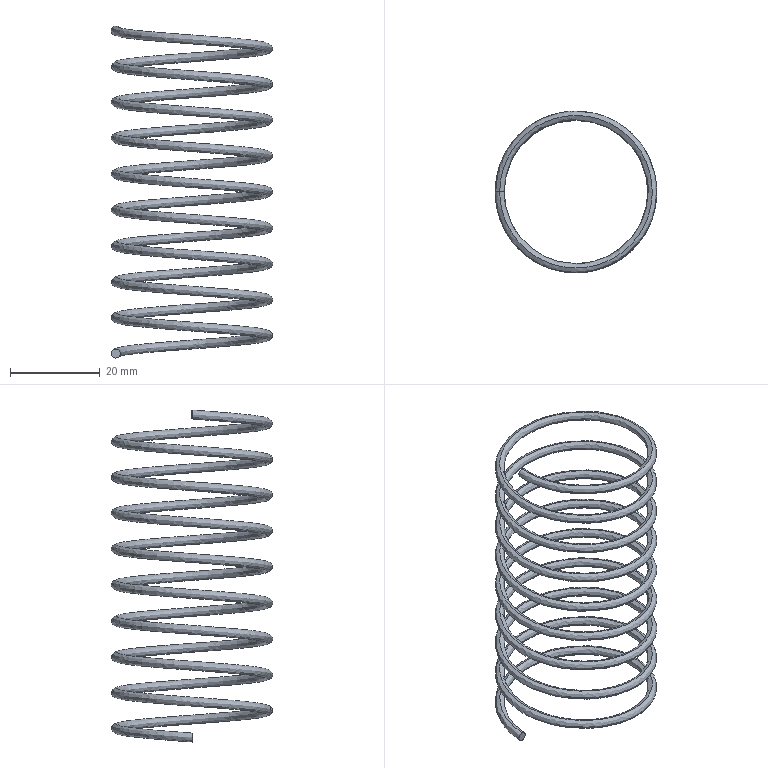Part | SolidWorks | features BaseBody 1 | 1 solid | 4 faces | box 36 x 36 x 74 mm | volume 3015 mm3 | plane 2 | spline 2